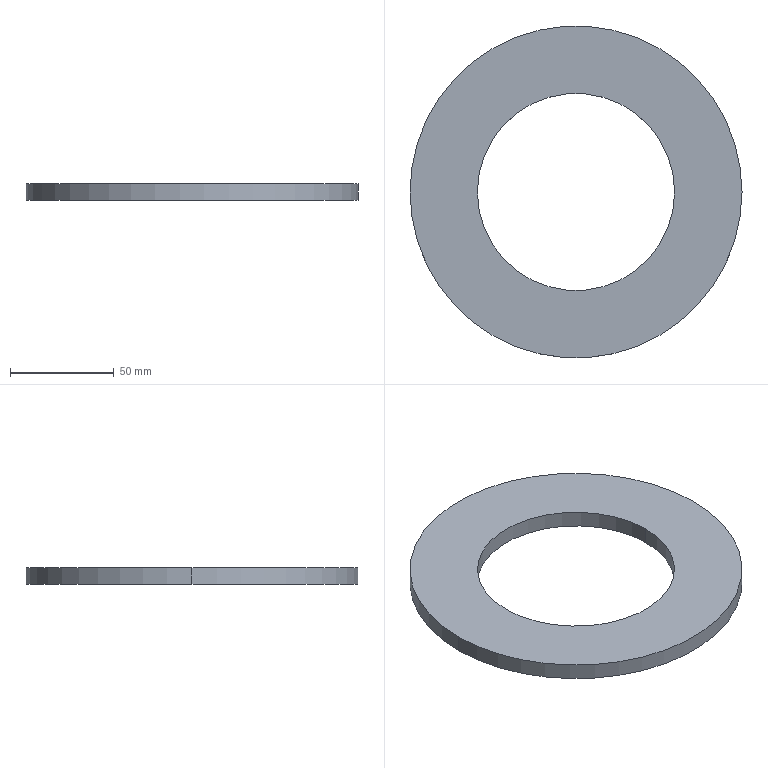Part | STEP file | Rubber pad_Default<As machined> | 1 solid | 6 faces | box 160 x 160 x 8 mm | volume 104144 mm3 | cylinder 4 | plane 2 | commonest cylinder face diameters 95 x2 160 x2
STEP:
#1=CARTESIAN_POINT('',(0.,0.,0.));
#2=DIRECTION('',(0.,0.,1.));
#3=DIRECTION('',(1.,0.,0.));
#4=AXIS2_PLACEMENT_3D('',#1,#2,#3);
#5=CARTESIAN_POINT('',(-47.5,0.,8.));
#6=VERTEX_POINT('',#5);
#7=CARTESIAN_POINT('',(-47.5,0.,0.));
#8=VERTEX_POINT('',#7);
#9=CARTESIAN_POINT('',(-47.5,0.,8.));
#10=DIRECTION('',(0.,0.,-1.));
#11=VECTOR('',#10,1.);
#12=LINE('',#9,#11);
#13=CARTESIAN_POINT('',(0.,0.,8.));
#14=DIRECTION('',(0.,0.,-1.));
#15=DIRECTION('',(-1.,0.,0.));
#16=AXIS2_PLACEMENT_3D('',#13,#14,#15);
#17=CYLINDRICAL_SURFACE('',#16,47.5);
#18=CARTESIAN_POINT('',(6.283,0.));
#19=DIRECTION('',(0.,1.));
#20=VECTOR('',#19,1.);
#21=LINE('',#18,#20);
#22=(GEOMETRIC_REPRESENTATION_CONTEXT(2)PARAMETRIC_REPRESENTATION_CONTEXT()REPRESENTATION_CONTEXT('',''));
#23=DEFINITIONAL_REPRESENTATION('',(#21),#22);
#24=PCURVE('',#17,#23);
#25=CARTESIAN_POINT('',(0.,0.,8.));
#26=DIRECTION('',(0.,0.,-1.));
#27=DIRECTION('',(-1.,0.,0.));
#28=AXIS2_PLACEMENT_3D('',#25,#26,#27);
#29=CYLINDRICAL_SURFACE('',#28,47.5);
#30=CARTESIAN_POINT('',(0.,0.));
#31=DIRECTION('',(0.,1.));
#32=VECTOR('',#31,1.);
#33=LINE('',#30,#32);
#34=(GEOMETRIC_REPRESENTATION_CONTEXT(2)PARAMETRIC_REPRESENTATION_CONTEXT()REPRESENTATION_CONTEXT('',''));
#35=DEFINITIONAL_REPRESENTATION('',(#33),#34);
#36=PCURVE('',#29,#35);
#37=SURFACE_CURVE('',#12,(#24,#36),.PCURVE_S1.);
#38=EDGE_CURVE('',#6,#8,#37,.T.);
#39=ORIENTED_EDGE('',*,*,#38,.T.);
#40=CARTESIAN_POINT('',(47.5,0.,0.));
#41=VERTEX_POINT('',#40);
#42=CARTESIAN_POINT('',(0.,0.,0.));
#43=DIRECTION('',(0.,0.,1.));
#44=DIRECTION('',(1.,0.,0.));
#45=AXIS2_PLACEMENT_3D('',#42,#43,#44);
#46=CIRCLE('',#45,47.5);
#47=CARTESIAN_POINT('',(9.425,8.));
#48=DIRECTION('',(-1.,0.));
#49=VECTOR('',#48,1.);
#50=LINE('',#47,#49);
#51=(GEOMETRIC_REPRESENTATION_CONTEXT(2)PARAMETRIC_REPRESENTATION_CONTEXT()REPRESENTATION_CONTEXT('',''));
#52=DEFINITIONAL_REPRESENTATION('',(#50),#51);
#53=PCURVE('',#17,#52);
#54=CARTESIAN_POINT('',(0.,0.,0.));
#55=DIRECTION('',(0.,0.,1.));
#56=DIRECTION('',(1.,0.,0.));
#57=AXIS2_PLACEMENT_3D('',#54,#55,#56);
#58=PLANE('',#57);
#59=CARTESIAN_POINT('',(0.,0.));
#60=DIRECTION('',(1.,0.));
#61=AXIS2_PLACEMENT_2D('',#59,#60);
#62=CIRCLE('',#61,47.5);
#63=(GEOMETRIC_REPRESENTATION_CONTEXT(2)PARAMETRIC_REPRESENTATION_CONTEXT()REPRESENTATION_CONTEXT('',''));
#64=DEFINITIONAL_REPRESENTATION('',(#62),#63);
#65=PCURVE('',#58,#64);
#66=SURFACE_CURVE('',#46,(#53,#65),.PCURVE_S1.);
#67=EDGE_CURVE('',#8,#41,#66,.T.);
#68=ORIENTED_EDGE('',*,*,#67,.T.);
#69=CARTESIAN_POINT('',(47.5,0.,8.));
#70=VERTEX_POINT('',#69);
#71=CARTESIAN_POINT('',(47.5,0.,8.));
#72=DIRECTION('',(0.,0.,-1.));
#73=VECTOR('',#72,1.);
#74=LINE('',#71,#73);
#75=CARTESIAN_POINT('',(3.142,0.));
#76=DIRECTION('',(0.,1.));
#77=VECTOR('',#76,1.);
#78=LINE('',#75,#77);
#79=(GEOMETRIC_REPRESENTATION_CONTEXT(2)PARAMETRIC_REPRESENTATION_CONTEXT()REPRESENTATION_CONTEXT('',''));
#80=DEFINITIONAL_REPRESENTATION('',(#78),#79);
#81=PCURVE('',#17,#80);
#82=CARTESIAN_POINT('',(3.142,0.));
#83=DIRECTION('',(0.,1.));
#84=VECTOR('',#83,1.);
#85=LINE('',#82,#84);
#86=(GEOMETRIC_REPRESENTATION_CONTEXT(2)PARAMETRIC_REPRESENTATION_CONTEXT()REPRESENTATION_CONTEXT('',''));
#87=DEFINITIONAL_REPRESENTATION('',(#85),#86);
#88=PCURVE('',#29,#87);
#89=SURFACE_CURVE('',#74,(#81,#88),.PCURVE_S1.);
#90=EDGE_CURVE('',#70,#41,#89,.T.);
#91=ORIENTED_EDGE('',*,*,#90,.F.);
#92=CARTESIAN_POINT('',(0.,0.,8.));
#93=DIRECTION('',(0.,0.,1.));
#94=DIRECTION('',(1.,0.,0.));
#95=AXIS2_PLACEMENT_3D('',#92,#93,#94);
#96=CIRCLE('',#95,47.5);
#97=CARTESIAN_POINT('',(9.425,0.));
#98=DIRECTION('',(-1.,0.));
#99=VECTOR('',#98,1.);
#100=LINE('',#97,#99);
#101=(GEOMETRIC_REPRESENTATION_CONTEXT(2)PARAMETRIC_REPRESENTATION_CONTEXT()REPRESENTATION_CONTEXT('',''));
#102=DEFINITIONAL_REPRESENTATION('',(#100),#101);
#103=PCURVE('',#17,#102);
#104=CARTESIAN_POINT('',(0.,0.,8.));
#105=DIRECTION('',(0.,0.,1.));
#106=DIRECTION('',(1.,0.,0.));
#107=AXIS2_PLACEMENT_3D('',#104,#105,#106);
#108=PLANE('',#107);
#109=CARTESIAN_POINT('',(0.,0.));
#110=DIRECTION('',(1.,0.));
#111=AXIS2_PLACEMENT_2D('',#109,#110);
#112=CIRCLE('',#111,47.5);
#113=(GEOMETRIC_REPRESENTATION_CONTEXT(2)PARAMETRIC_REPRESENTATION_CONTEXT()REPRESENTATION_CONTEXT('',''));
#114=DEFINITIONAL_REPRESENTATION('',(#112),#113);
#115=PCURVE('',#108,#114);
#116=SURFACE_CURVE('',#96,(#103,#115),.PCURVE_S1.);
#117=EDGE_CURVE('',#6,#70,#116,.T.);
#118=ORIENTED_EDGE('',*,*,#117,.F.);
#119=EDGE_LOOP('',(#39,#68,#91,#118));
#120=FACE_BOUND('',#119,.F.);
#121=ADVANCED_FACE('',(#120),#17,.F.);
#122=CARTESIAN_POINT('',(80.,0.,8.));
#123=VERTEX_POINT('',#122);
#124=CARTESIAN_POINT('',(-80.,0.,8.));
#125=VERTEX_POINT('',#124);
#126=CARTESIAN_POINT('',(0.,0.,8.));
#127=DIRECTION('',(0.,0.,1.));
#128=DIRECTION('',(1.,0.,0.));
#129=AXIS2_PLACEMENT_3D('',#126,#127,#128);
#130=CIRCLE('',#129,80.);
#131=CARTESIAN_POINT('',(0.,0.,8.));
#132=DIRECTION('',(0.,0.,-1.));
#133=DIRECTION('',(-1.,0.,0.));
#134=AXIS2_PLACEMENT_3D('',#131,#132,#133);
#135=CYLINDRICAL_SURFACE('',#134,80.);
#136=CARTESIAN_POINT('',(3.142,0.));
#137=DIRECTION('',(-1.,0.));
#138=VECTOR('',#137,1.);
#139=LINE('',#136,#138);
#140=(GEOMETRIC_REPRESENTATION_CONTEXT(2)PARAMETRIC_REPRESENTATION_CONTEXT()REPRESENTATION_CONTEXT('',''));
#141=DEFINITIONAL_REPRESENTATION('',(#139),#140);
#142=PCURVE('',#135,#141);
#143=CARTESIAN_POINT('',(0.,0.));
#144=DIRECTION('',(1.,0.));
#145=AXIS2_PLACEMENT_2D('',#143,#144);
#146=CIRCLE('',#145,80.);
#147=(GEOMETRIC_REPRESENTATION_CONTEXT(2)PARAMETRIC_REPRESENTATION_CONTEXT()REPRESENTATION_CONTEXT('',''));
#148=DEFINITIONAL_REPRESENTATION('',(#146),#147);
#149=PCURVE('',#108,#148);
#150=SURFACE_CURVE('',#130,(#142,#149),.PCURVE_S1.);
#151=EDGE_CURVE('',#123,#125,#150,.T.);
#152=ORIENTED_EDGE('',*,*,#151,.F.);
#153=CARTESIAN_POINT('',(80.,0.,0.));
#154=VERTEX_POINT('',#153);
#155=CARTESIAN_POINT('',(80.,0.,8.));
#156=DIRECTION('',(0.,0.,-1.));
#157=VECTOR('',#156,1.);
#158=LINE('',#155,#157);
#159=CARTESIAN_POINT('',(3.142,0.));
#160=DIRECTION('',(0.,1.));
#161=VECTOR('',#160,1.);
#162=LINE('',#159,#161);
#163=(GEOMETRIC_REPRESENTATION_CONTEXT(2)PARAMETRIC_REPRESENTATION_CONTEXT()REPRESENTATION_CONTEXT('',''));
#164=DEFINITIONAL_REPRESENTATION('',(#162),#163);
#165=PCURVE('',#135,#164);
#166=CARTESIAN_POINT('',(0.,0.,8.));
#167=DIRECTION('',(0.,0.,-1.));
#168=DIRECTION('',(-1.,0.,0.));
#169=AXIS2_PLACEMENT_3D('',#166,#167,#168);
#170=CYLINDRICAL_SURFACE('',#169,80.);
#171=CARTESIAN_POINT('',(3.142,0.));
#172=DIRECTION('',(0.,1.));
#173=VECTOR('',#172,1.);
#174=LINE('',#171,#173);
#175=(GEOMETRIC_REPRESENTATION_CONTEXT(2)PARAMETRIC_REPRESENTATION_CONTEXT()REPRESENTATION_CONTEXT('',''));
#176=DEFINITIONAL_REPRESENTATION('',(#174),#175);
#177=PCURVE('',#170,#176);
#178=SURFACE_CURVE('',#158,(#165,#177),.PCURVE_S1.);
#179=EDGE_CURVE('',#123,#154,#178,.T.);
#180=ORIENTED_EDGE('',*,*,#179,.T.);
#181=CARTESIAN_POINT('',(-80.,0.,0.));
#182=VERTEX_POINT('',#181);
#183=CARTESIAN_POINT('',(0.,0.,0.));
#184=DIRECTION('',(0.,0.,1.));
#185=DIRECTION('',(1.,0.,0.));
#186=AXIS2_PLACEMENT_3D('',#183,#184,#185);
#187=CIRCLE('',#186,80.);
#188=CARTESIAN_POINT('',(3.142,8.));
#189=DIRECTION('',(-1.,0.));
#190=VECTOR('',#189,1.);
#191=LINE('',#188,#190);
#192=(GEOMETRIC_REPRESENTATION_CONTEXT(2)PARAMETRIC_REPRESENTATION_CONTEXT()REPRESENTATION_CONTEXT('',''));
#193=DEFINITIONAL_REPRESENTATION('',(#191),#192);
#194=PCURVE('',#135,#193);
#195=CARTESIAN_POINT('',(0.,0.));
#196=DIRECTION('',(1.,0.));
#197=AXIS2_PLACEMENT_2D('',#195,#196);
#198=CIRCLE('',#197,80.);
#199=(GEOMETRIC_REPRESENTATION_CONTEXT(2)PARAMETRIC_REPRESENTATION_CONTEXT()REPRESENTATION_CONTEXT('',''));
#200=DEFINITIONAL_REPRESENTATION('',(#198),#199);
#201=PCURVE('',#58,#200);
#202=SURFACE_CURVE('',#187,(#194,#201),.PCURVE_S1.);
#203=EDGE_CURVE('',#154,#182,#202,.T.);
#204=ORIENTED_EDGE('',*,*,#203,.T.);
#205=CARTESIAN_POINT('',(-80.,0.,8.));
#206=DIRECTION('',(0.,0.,-1.));
#207=VECTOR('',#206,1.);
#208=LINE('',#205,#207);
#209=CARTESIAN_POINT('',(0.,0.));
#210=DIRECTION('',(0.,1.));
#211=VECTOR('',#210,1.);
#212=LINE('',#209,#211);
#213=(GEOMETRIC_REPRESENTATION_CONTEXT(2)PARAMETRIC_REPRESENTATION_CONTEXT()REPRESENTATION_CONTEXT('',''));
#214=DEFINITIONAL_REPRESENTATION('',(#212),#213);
#215=PCURVE('',#135,#214);
#216=CARTESIAN_POINT('',(6.283,0.));
#217=DIRECTION('',(0.,1.));
#218=VECTOR('',#217,1.);
#219=LINE('',#216,#218);
#220=(GEOMETRIC_REPRESENTATION_CONTEXT(2)PARAMETRIC_REPRESENTATION_CONTEXT()REPRESENTATION_CONTEXT('',''));
#221=DEFINITIONAL_REPRESENTATION('',(#219),#220);
#222=PCURVE('',#170,#221);
#223=SURFACE_CURVE('',#208,(#215,#222),.PCURVE_S1.);
#224=EDGE_CURVE('',#125,#182,#223,.T.);
#225=ORIENTED_EDGE('',*,*,#224,.F.);
#226=EDGE_LOOP('',(#152,#180,#204,#225));
#227=FACE_BOUND('',#226,.T.);
#228=ADVANCED_FACE('',(#227),#135,.T.);
#229=CARTESIAN_POINT('',(0.,0.,8.));
#230=DIRECTION('',(0.,0.,1.));
#231=DIRECTION('',(1.,0.,0.));
#232=AXIS2_PLACEMENT_3D('',#229,#230,#231);
#233=CIRCLE('',#232,80.);
#234=CARTESIAN_POINT('',(0.,0.));
#235=DIRECTION('',(1.,0.));
#236=AXIS2_PLACEMENT_2D('',#234,#235);
#237=CIRCLE('',#236,80.);
#238=(GEOMETRIC_REPRESENTATION_CONTEXT(2)PARAMETRIC_REPRESENTATION_CONTEXT()REPRESENTATION_CONTEXT('',''));
#239=DEFINITIONAL_REPRESENTATION('',(#237),#238);
#240=PCURVE('',#108,#239);
#241=CARTESIAN_POINT('',(9.425,0.));
#242=DIRECTION('',(-1.,0.));
#243=VECTOR('',#242,1.);
#244=LINE('',#241,#243);
#245=(GEOMETRIC_REPRESENTATION_CONTEXT(2)PARAMETRIC_REPRESENTATION_CONTEXT()REPRESENTATION_CONTEXT('',''));
#246=DEFINITIONAL_REPRESENTATION('',(#244),#245);
#247=PCURVE('',#170,#246);
#248=SURFACE_CURVE('',#233,(#240,#247),.PCURVE_S1.);
#249=EDGE_CURVE('',#125,#123,#248,.T.);
#250=ORIENTED_EDGE('',*,*,#249,.T.);
#251=ORIENTED_EDGE('',*,*,#151,.T.);
#252=EDGE_LOOP('',(#250,#251));
#253=FACE_BOUND('',#252,.T.);
#254=ORIENTED_EDGE('',*,*,#117,.F.);
#255=CARTESIAN_POINT('',(0.,0.,8.));
#256=DIRECTION('',(0.,0.,1.));
#257=DIRECTION('',(1.,0.,0.));
#258=AXIS2_PLACEMENT_3D('',#255,#256,#257);
#259=CIRCLE('',#258,47.5);
#260=CARTESIAN_POINT('',(0.,0.));
#261=DIRECTION('',(1.,0.));
#262=AXIS2_PLACEMENT_2D('',#260,#261);
#263=CIRCLE('',#262,47.5);
#264=(GEOMETRIC_REPRESENTATION_CONTEXT(2)PARAMETRIC_REPRESENTATION_CONTEXT()REPRESENTATION_CONTEXT('',''));
#265=DEFINITIONAL_REPRESENTATION('',(#263),#264);
#266=PCURVE('',#108,#265);
#267=CARTESIAN_POINT('',(3.142,0.));
#268=DIRECTION('',(-1.,0.));
#269=VECTOR('',#268,1.);
#270=LINE('',#267,#269);
#271=(GEOMETRIC_REPRESENTATION_CONTEXT(2)PARAMETRIC_REPRESENTATION_CONTEXT()REPRESENTATION_CONTEXT('',''));
#272=DEFINITIONAL_REPRESENTATION('',(#270),#271);
#273=PCURVE('',#29,#272);
#274=SURFACE_CURVE('',#259,(#266,#273),.PCURVE_S1.);
#275=EDGE_CURVE('',#70,#6,#274,.T.);
#276=ORIENTED_EDGE('',*,*,#275,.F.);
#277=EDGE_LOOP('',(#254,#276));
#278=FACE_BOUND('',#277,.T.);
#279=ADVANCED_FACE('',(#253,#278),#108,.T.);
#280=CARTESIAN_POINT('',(0.,0.,0.));
#281=DIRECTION('',(0.,0.,1.));
#282=DIRECTION('',(1.,0.,0.));
#283=AXIS2_PLACEMENT_3D('',#280,#281,#282);
#284=CIRCLE('',#283,80.);
#285=CARTESIAN_POINT('',(0.,0.));
#286=DIRECTION('',(1.,0.));
#287=AXIS2_PLACEMENT_2D('',#285,#286);
#288=CIRCLE('',#287,80.);
#289=(GEOMETRIC_REPRESENTATION_CONTEXT(2)PARAMETRIC_REPRESENTATION_CONTEXT()REPRESENTATION_CONTEXT('',''));
#290=DEFINITIONAL_REPRESENTATION('',(#288),#289);
#291=PCURVE('',#58,#290);
#292=CARTESIAN_POINT('',(9.425,8.));
#293=DIRECTION('',(-1.,0.));
#294=VECTOR('',#293,1.);
#295=LINE('',#292,#294);
#296=(GEOMETRIC_REPRESENTATION_CONTEXT(2)PARAMETRIC_REPRESENTATION_CONTEXT()REPRESENTATION_CONTEXT('',''));
#297=DEFINITIONAL_REPRESENTATION('',(#295),#296);
#298=PCURVE('',#170,#297);
#299=SURFACE_CURVE('',#284,(#291,#298),.PCURVE_S1.);
#300=EDGE_CURVE('',#182,#154,#299,.T.);
#301=ORIENTED_EDGE('',*,*,#300,.F.);
#302=ORIENTED_EDGE('',*,*,#203,.F.);
#303=EDGE_LOOP('',(#301,#302));
#304=FACE_BOUND('',#303,.T.);
#305=ORIENTED_EDGE('',*,*,#67,.T.);
#306=CARTESIAN_POINT('',(0.,0.,0.));
#307=DIRECTION('',(0.,0.,1.));
#308=DIRECTION('',(1.,0.,0.));
#309=AXIS2_PLACEMENT_3D('',#306,#307,#308);
#310=CIRCLE('',#309,47.5);
#311=CARTESIAN_POINT('',(0.,0.));
#312=DIRECTION('',(1.,0.));
#313=AXIS2_PLACEMENT_2D('',#311,#312);
#314=CIRCLE('',#313,47.5);
#315=(GEOMETRIC_REPRESENTATION_CONTEXT(2)PARAMETRIC_REPRESENTATION_CONTEXT()REPRESENTATION_CONTEXT('',''));
#316=DEFINITIONAL_REPRESENTATION('',(#314),#315);
#317=PCURVE('',#58,#316);
#318=CARTESIAN_POINT('',(3.142,8.));
#319=DIRECTION('',(-1.,0.));
#320=VECTOR('',#319,1.);
#321=LINE('',#318,#320);
#322=(GEOMETRIC_REPRESENTATION_CONTEXT(2)PARAMETRIC_REPRESENTATION_CONTEXT()REPRESENTATION_CONTEXT('',''));
#323=DEFINITIONAL_REPRESENTATION('',(#321),#322);
#324=PCURVE('',#29,#323);
#325=SURFACE_CURVE('',#310,(#317,#324),.PCURVE_S1.);
#326=EDGE_CURVE('',#41,#8,#325,.T.);
#327=ORIENTED_EDGE('',*,*,#326,.T.);
#328=EDGE_LOOP('',(#305,#327));
#329=FACE_BOUND('',#328,.T.);
#330=ADVANCED_FACE('',(#304,#329),#58,.F.);
#331=ORIENTED_EDGE('',*,*,#179,.F.);
#332=ORIENTED_EDGE('',*,*,#249,.F.);
#333=ORIENTED_EDGE('',*,*,#224,.T.);
#334=ORIENTED_EDGE('',*,*,#300,.T.);
#335=EDGE_LOOP('',(#331,#332,#333,#334));
#336=FACE_BOUND('',#335,.T.);
#337=ADVANCED_FACE('',(#336),#170,.T.);
#338=ORIENTED_EDGE('',*,*,#326,.T.);
#339=ORIENTED_EDGE('',*,*,#38,.F.);
#340=ORIENTED_EDGE('',*,*,#275,.F.);
#341=ORIENTED_EDGE('',*,*,#90,.T.);
#342=EDGE_LOOP('',(#338,#339,#340,#341));
#343=FACE_BOUND('',#342,.F.);
#344=ADVANCED_FACE('',(#343),#29,.F.);
#345=CLOSED_SHELL('',(#121,#228,#279,#330,#337,#344));
#346=MANIFOLD_SOLID_BREP('',#345);
#347=(LENGTH_UNIT()NAMED_UNIT(*)SI_UNIT(.MILLI.,.METRE.));
#348=UNCERTAINTY_MEASURE_WITH_UNIT(LENGTH_MEASURE(0.0000001),#347,'','');
#349=(NAMED_UNIT(*)PLANE_ANGLE_UNIT()SI_UNIT($,.RADIAN.));
#350=(NAMED_UNIT(*)SI_UNIT($,.STERADIAN.)SOLID_ANGLE_UNIT());
#351=(GEOMETRIC_REPRESENTATION_CONTEXT(3)GLOBAL_UNCERTAINTY_ASSIGNED_CONTEXT((#348))GLOBAL_UNIT_ASSIGNED_CONTEXT((#347,#349,#350))REPRESENTATION_CONTEXT('',''));
#352=ADVANCED_BREP_SHAPE_REPRESENTATION('',(#4,#346),#351);